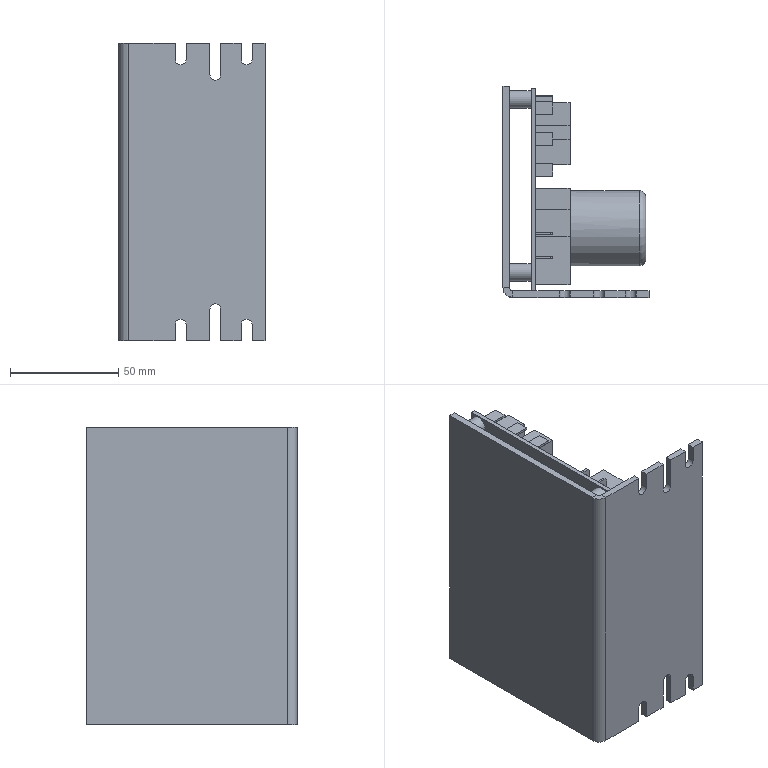Part | STEP file | ZYXK6.1012.V1.1 | 1 solid | 169 faces | box 67.5 x 97.5 x 137.5 mm | volume 163388 mm3 | plane 151 | cylinder 17 | torus 1 | commonest cylinder face diameters 5 x6 2 x4 8 x4 3 x1 9 x1 35 x1